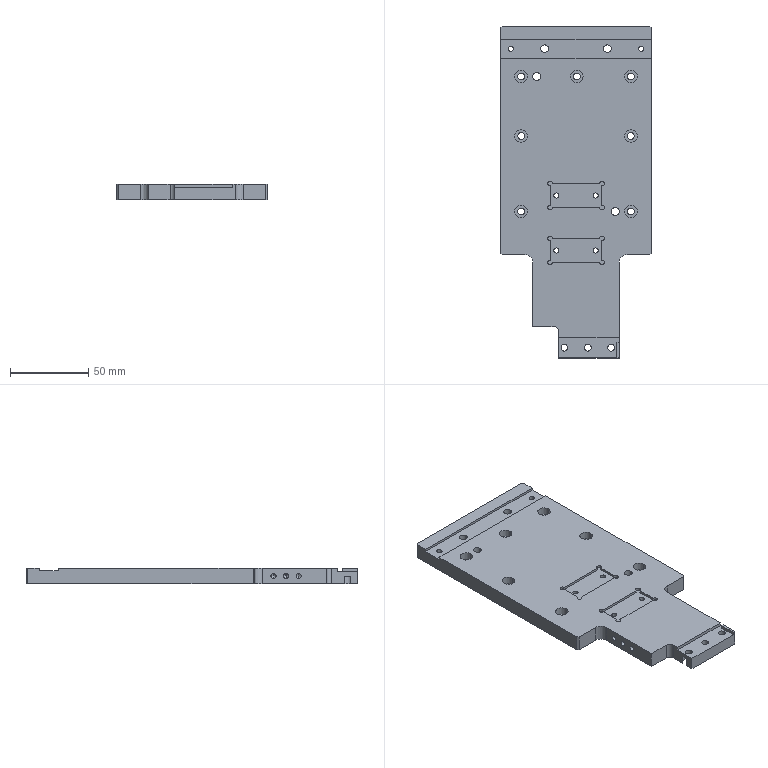Part | SolidWorks | features ICE 21, HoleWzd 16, Fillet 5, MoveFace 3, LPattern 2, MirrorPattern 2, Chamfer 1, Extrusion 1 | 1 solid | 143 faces | box 96 x 211.5 x 10 mm | volume 163638 mm3 | cylinder 86 | plane 45 | cone 12 | commonest cylinder face diameters 3.3 x24 8 x19 4.4 x14 3 x12 5 x8 4.3 x6